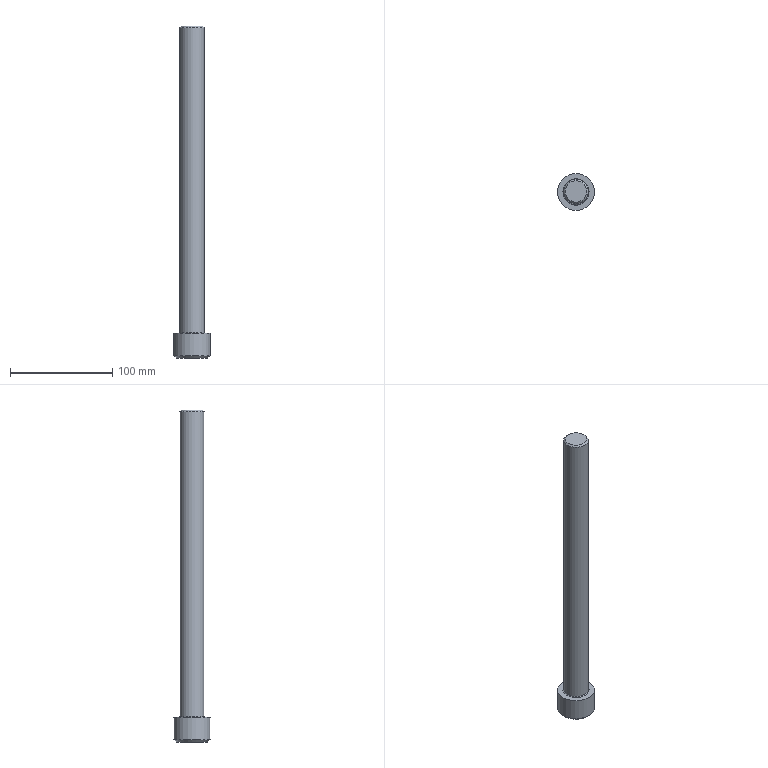Part | STEP file | solid 12 | 1 solid | 21 faces | box 36 x 36 x 324 mm | volume 155996 mm3 | plane 10 | sphere 6 | cylinder 2 | cone 2 | torus 1 | commonest cylinder face diameters 24 x1 36 x1